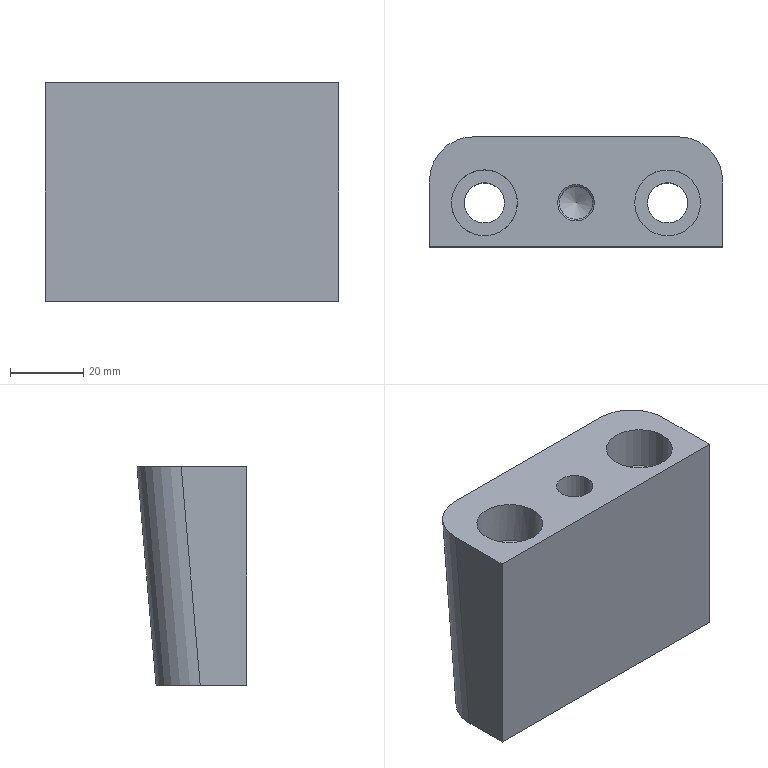Part | STEP file | solid 132 | 1 solid | 18 faces | box 80 x 30 x 59.496 mm | volume 109836 mm3 | plane 8 | cylinder 8 | cone 2 | commonest cylinder face diameters 11 x2 18 x2 24 x2 9 x1 10 x1